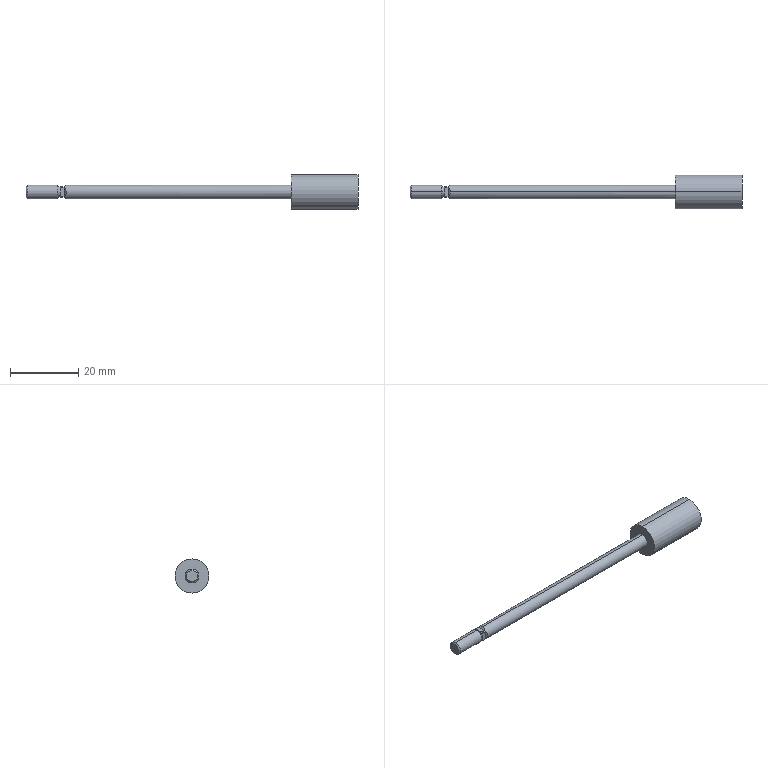Part | SolidWorks | features RefAxis 6, ICE 4, 3DProfileFeature 2, Revolution 1, Scale 1 | 1 solid | 30 faces | box 97.25 x 10 x 10 mm | volume 2498 mm3 | plane 16 | cylinder 8 | cone 6 | commonest cylinder face diameters 4 x4 3 x2 10 x2
STEP:
#1=CARTESIAN_POINT('',(126.058,0.000000064,5.));
#2=VERTEX_POINT('',#1);
#3=CARTESIAN_POINT('',(126.058,0.000000064,-5.));
#4=VERTEX_POINT('',#3);
#5=CARTESIAN_POINT('',(126.058,0.000000064,0.000001901));
#6=DIRECTION('',(-1.,0.,0.));
#7=DIRECTION('',(0.,0.,1.));
#8=AXIS2_PLACEMENT_3D('',#5,#6,#7);
#9=CIRCLE('',#8,5.);
#10=EDGE_CURVE('',#2,#4,#9,.T.);
#11=ORIENTED_EDGE('',*,*,#10,.T.);
#12=CARTESIAN_POINT('',(106.558,0.000000064,-5.));
#13=VERTEX_POINT('',#12);
#14=CARTESIAN_POINT('',(126.058,0.000000064,-5.));
#15=DIRECTION('',(-1.,0.,0.));
#16=VECTOR('',#15,1000.);
#17=LINE('',#14,#16);
#18=EDGE_CURVE('',#4,#13,#17,.T.);
#19=ORIENTED_EDGE('',*,*,#18,.T.);
#20=CARTESIAN_POINT('',(106.558,0.000000064,5.));
#21=VERTEX_POINT('',#20);
#22=CARTESIAN_POINT('',(106.558,0.000000064,0.000001901));
#23=DIRECTION('',(-1.,0.,0.));
#24=DIRECTION('',(0.,0.,1.));
#25=AXIS2_PLACEMENT_3D('',#22,#23,#24);
#26=CIRCLE('',#25,5.);
#27=EDGE_CURVE('',#21,#13,#26,.T.);
#28=ORIENTED_EDGE('',*,*,#27,.F.);
#29=CARTESIAN_POINT('',(126.058,0.000000064,5.));
#30=DIRECTION('',(-1.,0.,0.));
#31=VECTOR('',#30,1000.);
#32=LINE('',#29,#31);
#33=EDGE_CURVE('',#2,#21,#32,.T.);
#34=ORIENTED_EDGE('',*,*,#33,.F.);
#35=EDGE_LOOP('',(#11,#19,#28,#34));
#36=FACE_OUTER_BOUND('',#35,.T.);
#37=CARTESIAN_POINT('',(126.058,0.000000064,0.000001901));
#38=DIRECTION('',(-1.,0.,0.));
#39=DIRECTION('',(0.,0.,1.));
#40=AXIS2_PLACEMENT_3D('',#37,#38,#39);
#41=CYLINDRICAL_SURFACE('',#40,5.);
#42=ADVANCED_FACE('',(#36),#41,.T.);
#43=CARTESIAN_POINT('',(106.558,0.000000064,2.));
#44=VERTEX_POINT('',#43);
#45=CARTESIAN_POINT('',(106.558,0.000000064,-2.));
#46=VERTEX_POINT('',#45);
#47=CARTESIAN_POINT('',(106.558,0.000000064,0.000001901));
#48=DIRECTION('',(-1.,0.,0.));
#49=DIRECTION('',(0.,0.,1.));
#50=AXIS2_PLACEMENT_3D('',#47,#48,#49);
#51=CIRCLE('',#50,2.);
#52=EDGE_CURVE('',#44,#46,#51,.T.);
#53=ORIENTED_EDGE('',*,*,#52,.T.);
#54=CARTESIAN_POINT('',(40.558,0.000000064,-2.));
#55=VERTEX_POINT('',#54);
#56=CARTESIAN_POINT('',(126.058,0.000000064,-2.));
#57=DIRECTION('',(-1.,0.,0.));
#58=VECTOR('',#57,1000.);
#59=LINE('',#56,#58);
#60=EDGE_CURVE('',#46,#55,#59,.T.);
#61=ORIENTED_EDGE('',*,*,#60,.T.);
#62=CARTESIAN_POINT('',(40.058,1.323,-1.5));
#63=VERTEX_POINT('',#62);
#64=CARTESIAN_POINT('',(40.558,0.000000064,-2.));
#65=CARTESIAN_POINT('',(40.558,0.4926,-2.));
#66=CARTESIAN_POINT('',(40.384,0.9534,-1.826));
#67=CARTESIAN_POINT('',(40.058,1.323,-1.5));
#68=(BOUNDED_CURVE()B_SPLINE_CURVE(3,(#64,#65,#66,#67),.UNSPECIFIED.,.F.,.F.)B_SPLINE_CURVE_WITH_KNOTS((4,4),(3.142,3.864),.UNSPECIFIED.)CURVE()GEOMETRIC_REPRESENTATION_ITEM()RATIONAL_B_SPLINE_CURVE((1.,0.9569,0.9569,1.))REPRESENTATION_ITEM(''));
#69=EDGE_CURVE('',#55,#63,#68,.T.);
#70=ORIENTED_EDGE('',*,*,#69,.T.);
#71=CARTESIAN_POINT('',(39.183,1.323,-1.5));
#72=VERTEX_POINT('',#71);
#73=CARTESIAN_POINT('',(126.058,1.323,-1.5));
#74=DIRECTION('',(-1.,0.,0.));
#75=VECTOR('',#74,1000.);
#76=LINE('',#73,#75);
#77=EDGE_CURVE('',#63,#72,#76,.T.);
#78=ORIENTED_EDGE('',*,*,#77,.T.);
#79=CARTESIAN_POINT('',(39.183,1.5,-1.323));
#80=VERTEX_POINT('',#79);
#81=CARTESIAN_POINT('',(39.183,0.000000064,0.000001901));
#82=DIRECTION('',(-1.,0.,0.));
#83=DIRECTION('',(0.,0.,1.));
#84=AXIS2_PLACEMENT_3D('',#81,#82,#83);
#85=CIRCLE('',#84,2.);
#86=EDGE_CURVE('',#80,#72,#85,.T.);
#87=ORIENTED_EDGE('',*,*,#86,.F.);
#88=CARTESIAN_POINT('',(40.058,1.5,-1.323));
#89=VERTEX_POINT('',#88);
#90=CARTESIAN_POINT('',(126.058,1.5,-1.323));
#91=DIRECTION('',(1.,0.,0.));
#92=VECTOR('',#91,1000.);
#93=LINE('',#90,#92);
#94=EDGE_CURVE('',#80,#89,#93,.T.);
#95=ORIENTED_EDGE('',*,*,#94,.T.);
#96=CARTESIAN_POINT('',(40.058,1.5,1.323));
#97=VERTEX_POINT('',#96);
#98=CARTESIAN_POINT('',(40.058,1.5,-1.323));
#99=CARTESIAN_POINT('',(40.758,2.2,-0.5291));
#100=CARTESIAN_POINT('',(40.758,2.2,0.5292));
#101=CARTESIAN_POINT('',(40.058,1.5,1.323));
#102=(BOUNDED_CURVE()B_SPLINE_CURVE(3,(#98,#99,#100,#101),.UNSPECIFIED.,.F.,.F.)B_SPLINE_CURVE_WITH_KNOTS((4,4),(2.419,3.864),.UNSPECIFIED.)CURVE()GEOMETRIC_REPRESENTATION_ITEM()RATIONAL_B_SPLINE_CURVE((1.,0.8333,0.8333,1.))REPRESENTATION_ITEM(''));
#103=EDGE_CURVE('',#89,#97,#102,.T.);
#104=ORIENTED_EDGE('',*,*,#103,.T.);
#105=CARTESIAN_POINT('',(39.183,1.5,1.323));
#106=VERTEX_POINT('',#105);
#107=CARTESIAN_POINT('',(126.058,1.5,1.323));
#108=DIRECTION('',(-1.,0.,0.));
#109=VECTOR('',#108,1000.);
#110=LINE('',#107,#109);
#111=EDGE_CURVE('',#97,#106,#110,.T.);
#112=ORIENTED_EDGE('',*,*,#111,.T.);
#113=CARTESIAN_POINT('',(39.183,1.323,1.5));
#114=VERTEX_POINT('',#113);
#115=CARTESIAN_POINT('',(39.183,0.000000064,0.000001901));
#116=DIRECTION('',(-1.,0.,0.));
#117=DIRECTION('',(0.,0.,1.));
#118=AXIS2_PLACEMENT_3D('',#115,#116,#117);
#119=CIRCLE('',#118,2.);
#120=EDGE_CURVE('',#114,#106,#119,.T.);
#121=ORIENTED_EDGE('',*,*,#120,.F.);
#122=CARTESIAN_POINT('',(40.058,1.323,1.5));
#123=VERTEX_POINT('',#122);
#124=CARTESIAN_POINT('',(126.058,1.323,1.5));
#125=DIRECTION('',(1.,0.,0.));
#126=VECTOR('',#125,1000.);
#127=LINE('',#124,#126);
#128=EDGE_CURVE('',#114,#123,#127,.T.);
#129=ORIENTED_EDGE('',*,*,#128,.T.);
#130=CARTESIAN_POINT('',(40.558,0.000000064,2.));
#131=VERTEX_POINT('',#130);
#132=CARTESIAN_POINT('',(40.058,1.323,1.5));
#133=CARTESIAN_POINT('',(40.384,0.9534,1.826));
#134=CARTESIAN_POINT('',(40.558,0.4926,2.));
#135=CARTESIAN_POINT('',(40.558,0.000000064,2.));
#136=(BOUNDED_CURVE()B_SPLINE_CURVE(3,(#132,#133,#134,#135),.UNSPECIFIED.,.F.,.F.)B_SPLINE_CURVE_WITH_KNOTS((4,4),(2.419,3.142),.UNSPECIFIED.)CURVE()GEOMETRIC_REPRESENTATION_ITEM()RATIONAL_B_SPLINE_CURVE((1.,0.9569,0.9569,1.))REPRESENTATION_ITEM(''));
#137=EDGE_CURVE('',#123,#131,#136,.T.);
#138=ORIENTED_EDGE('',*,*,#137,.T.);
#139=CARTESIAN_POINT('',(126.058,0.000000064,2.));
#140=DIRECTION('',(-1.,0.,0.));
#141=VECTOR('',#140,1000.);
#142=LINE('',#139,#141);
#143=EDGE_CURVE('',#44,#131,#142,.T.);
#144=ORIENTED_EDGE('',*,*,#143,.F.);
#145=EDGE_LOOP('',(#53,#61,#70,#78,#87,#95,#104,#112,#121,#129,#138,#144));
#146=FACE_OUTER_BOUND('',#145,.T.);
#147=CARTESIAN_POINT('',(126.058,0.000000064,0.000001901));
#148=DIRECTION('',(-1.,0.,0.));
#149=DIRECTION('',(0.,0.,1.));
#150=AXIS2_PLACEMENT_3D('',#147,#148,#149);
#151=CYLINDRICAL_SURFACE('',#150,2.);
#152=ADVANCED_FACE('',(#146),#151,.T.);
#153=CARTESIAN_POINT('',(38.808,1.5,0.000001901));
#154=VERTEX_POINT('',#153);
#155=CARTESIAN_POINT('',(38.808,0.000000064,-1.5));
#156=VERTEX_POINT('',#155);
#157=CARTESIAN_POINT('',(38.808,0.000000064,0.000001901));
#158=DIRECTION('',(-1.,0.,0.));
#159=DIRECTION('',(0.,0.,1.));
#160=AXIS2_PLACEMENT_3D('',#157,#158,#159);
#161=CIRCLE('',#160,1.5);
#162=EDGE_CURVE('',#154,#156,#161,.T.);
#163=ORIENTED_EDGE('',*,*,#162,.T.);
#164=CARTESIAN_POINT('',(38.058,0.000000064,-1.5));
#165=VERTEX_POINT('',#164);
#166=CARTESIAN_POINT('',(126.058,0.000000064,-1.5));
#167=DIRECTION('',(-1.,0.,0.));
#168=VECTOR('',#167,1000.);
#169=LINE('',#166,#168);
#170=EDGE_CURVE('',#156,#165,#169,.T.);
#171=ORIENTED_EDGE('',*,*,#170,.T.);
#172=CARTESIAN_POINT('',(38.058,0.000000064,1.5));
#173=VERTEX_POINT('',#172);
#174=CARTESIAN_POINT('',(38.058,0.000000064,0.000001901));
#175=DIRECTION('',(-1.,0.,0.));
#176=DIRECTION('',(0.,0.,1.));
#177=AXIS2_PLACEMENT_3D('',#174,#175,#176);
#178=CIRCLE('',#177,1.5);
#179=EDGE_CURVE('',#173,#165,#178,.T.);
#180=ORIENTED_EDGE('',*,*,#179,.F.);
#181=CARTESIAN_POINT('',(38.808,0.000000064,1.5));
#182=VERTEX_POINT('',#181);
#183=CARTESIAN_POINT('',(126.058,0.000000064,1.5));
#184=DIRECTION('',(-1.,0.,0.));
#185=VECTOR('',#184,1000.);
#186=LINE('',#183,#185);
#187=EDGE_CURVE('',#182,#173,#186,.T.);
#188=ORIENTED_EDGE('',*,*,#187,.F.);
#189=CARTESIAN_POINT('',(38.808,0.000000064,0.000001901));
#190=DIRECTION('',(-1.,0.,0.));
#191=DIRECTION('',(0.,0.,1.));
#192=AXIS2_PLACEMENT_3D('',#189,#190,#191);
#193=CIRCLE('',#192,1.5);
#194=EDGE_CURVE('',#182,#154,#193,.T.);
#195=ORIENTED_EDGE('',*,*,#194,.T.);
#196=EDGE_LOOP('',(#163,#171,#180,#188,#195));
#197=FACE_OUTER_BOUND('',#196,.T.);
#198=CARTESIAN_POINT('',(126.058,0.000000064,0.000001901));
#199=DIRECTION('',(-1.,0.,0.));
#200=DIRECTION('',(0.,0.,1.));
#201=AXIS2_PLACEMENT_3D('',#198,#199,#200);
#202=CYLINDRICAL_SURFACE('',#201,1.5);
#203=ADVANCED_FACE('',(#197),#202,.T.);
#204=CARTESIAN_POINT('',(38.058,0.000000064,2.));
#205=VERTEX_POINT('',#204);
#206=CARTESIAN_POINT('',(38.058,0.000000064,-2.));
#207=VERTEX_POINT('',#206);
#208=CARTESIAN_POINT('',(38.058,0.000000064,0.000001901));
#209=DIRECTION('',(-1.,0.,0.));
#210=DIRECTION('',(0.,0.,1.));
#211=AXIS2_PLACEMENT_3D('',#208,#209,#210);
#212=CIRCLE('',#211,2.);
#213=EDGE_CURVE('',#205,#207,#212,.T.);
#214=ORIENTED_EDGE('',*,*,#213,.T.);
#215=CARTESIAN_POINT('',(29.192,0.000000064,-2.));
#216=VERTEX_POINT('',#215);
#217=CARTESIAN_POINT('',(126.058,0.000000064,-2.));
#218=DIRECTION('',(-1.,0.,0.));
#219=VECTOR('',#218,1000.);
#220=LINE('',#217,#219);
#221=EDGE_CURVE('',#207,#216,#220,.T.);
#222=ORIENTED_EDGE('',*,*,#221,.T.);
#223=CARTESIAN_POINT('',(29.192,0.000000064,2.));
#224=VERTEX_POINT('',#223);
#225=CARTESIAN_POINT('',(29.192,0.000000064,0.000001901));
#226=DIRECTION('',(-1.,0.,0.));
#227=DIRECTION('',(0.,0.,1.));
#228=AXIS2_PLACEMENT_3D('',#225,#226,#227);
#229=CIRCLE('',#228,2.);
#230=EDGE_CURVE('',#224,#216,#229,.T.);
#231=ORIENTED_EDGE('',*,*,#230,.F.);
#232=CARTESIAN_POINT('',(126.058,0.000000064,2.));
#233=DIRECTION('',(-1.,0.,0.));
#234=VECTOR('',#233,1000.);
#235=LINE('',#232,#234);
#236=EDGE_CURVE('',#205,#224,#235,.T.);
#237=ORIENTED_EDGE('',*,*,#236,.F.);
#238=EDGE_LOOP('',(#214,#222,#231,#237));
#239=FACE_OUTER_BOUND('',#238,.T.);
#240=CARTESIAN_POINT('',(126.058,0.000000064,0.000001901));
#241=DIRECTION('',(-1.,0.,0.));
#242=DIRECTION('',(0.,0.,1.));
#243=AXIS2_PLACEMENT_3D('',#240,#241,#242);
#244=CYLINDRICAL_SURFACE('',#243,2.);
#245=ADVANCED_FACE('',(#239),#244,.T.);
#246=CARTESIAN_POINT('',(28.808,0.000000064,1.617));
#247=VERTEX_POINT('',#246);
#248=CARTESIAN_POINT('',(28.808,0.000000064,-1.616));
#249=VERTEX_POINT('',#248);
#250=CARTESIAN_POINT('',(28.808,0.000000064,0.000001901));
#251=DIRECTION('',(-1.,0.,0.));
#252=DIRECTION('',(0.,0.,1.));
#253=AXIS2_PLACEMENT_3D('',#250,#251,#252);
#254=CIRCLE('',#253,1.617);
#255=EDGE_CURVE('',#247,#249,#254,.T.);
#256=ORIENTED_EDGE('',*,*,#255,.F.);
#257=CARTESIAN_POINT('',(29.192,0.000000064,2.));
#258=DIRECTION('',(0.7071,0.,0.7071));
#259=VECTOR('',#258,1000.);
#260=LINE('',#257,#259);
#261=EDGE_CURVE('',#247,#224,#260,.T.);
#262=ORIENTED_EDGE('',*,*,#261,.T.);
#263=ORIENTED_EDGE('',*,*,#230,.T.);
#264=CARTESIAN_POINT('',(29.192,0.000000064,-2.));
#265=DIRECTION('',(0.7071,0.,-0.7071));
#266=VECTOR('',#265,1000.);
#267=LINE('',#264,#266);
#268=EDGE_CURVE('',#249,#216,#267,.T.);
#269=ORIENTED_EDGE('',*,*,#268,.F.);
#270=EDGE_LOOP('',(#256,#262,#263,#269));
#271=FACE_OUTER_BOUND('',#270,.T.);
#272=CARTESIAN_POINT('',(29.192,0.000000064,0.000001901));
#273=DIRECTION('',(1.,0.,0.));
#274=DIRECTION('',(0.,0.,-1.));
#275=AXIS2_PLACEMENT_3D('',#272,#273,#274);
#276=CONICAL_SURFACE('',#275,2.,0.7854);
#277=ADVANCED_FACE('',(#271),#276,.T.);
#278=CARTESIAN_POINT('',(38.808,-1.5,0.625));
#279=VERTEX_POINT('',#278);
#280=CARTESIAN_POINT('',(38.808,-0.625,1.5));
#281=VERTEX_POINT('',#280);
#282=CARTESIAN_POINT('',(38.808,0.000000064,0.000001901));
#283=DIRECTION('',(-1.,0.,0.));
#284=DIRECTION('',(0.,0.,1.));
#285=AXIS2_PLACEMENT_3D('',#282,#283,#284);
#286=CIRCLE('',#285,1.625);
#287=EDGE_CURVE('',#279,#281,#286,.T.);
#288=ORIENTED_EDGE('',*,*,#287,.T.);
#289=CARTESIAN_POINT('',(38.808,-2.,1.5));
#290=DIRECTION('',(0.,1.,0.));
#291=VECTOR('',#290,1000.);
#292=LINE('',#289,#291);
#293=EDGE_CURVE('',#281,#182,#292,.T.);
#294=ORIENTED_EDGE('',*,*,#293,.T.);
#295=CARTESIAN_POINT('',(38.808,-1.5,0.000001901));
#296=VERTEX_POINT('',#295);
#297=CARTESIAN_POINT('',(38.808,0.000000064,0.000001901));
#298=DIRECTION('',(-1.,0.,0.));
#299=DIRECTION('',(0.,0.,1.));
#300=AXIS2_PLACEMENT_3D('',#297,#298,#299);
#301=CIRCLE('',#300,1.5);
#302=EDGE_CURVE('',#296,#182,#301,.T.);
#303=ORIENTED_EDGE('',*,*,#302,.F.);
#304=CARTESIAN_POINT('',(38.808,-1.5,-2.));
#305=DIRECTION('',(0.,0.,1.));
#306=VECTOR('',#305,1000.);
#307=LINE('',#304,#306);
#308=EDGE_CURVE('',#296,#279,#307,.T.);
#309=ORIENTED_EDGE('',*,*,#308,.T.);
#310=EDGE_LOOP('',(#288,#294,#303,#309));
#311=FACE_OUTER_BOUND('',#310,.T.);
#312=CARTESIAN_POINT('',(38.808,1.5,0.000001901));
#313=DIRECTION('',(1.,0.,0.));
#314=DIRECTION('',(0.,0.,-1.));
#315=AXIS2_PLACEMENT_3D('',#312,#313,#314);
#316=PLANE('',#315);
#317=ADVANCED_FACE('',(#311),#316,.F.);
#318=CARTESIAN_POINT('',(39.183,-1.5,1.323));
#319=VERTEX_POINT('',#318);
#320=CARTESIAN_POINT('',(39.183,-1.323,1.5));
#321=VERTEX_POINT('',#320);
#322=CARTESIAN_POINT('',(39.183,0.000000064,0.000001901));
#323=DIRECTION('',(-1.,0.,0.));
#324=DIRECTION('',(0.,0.,1.));
#325=AXIS2_PLACEMENT_3D('',#322,#323,#324);
#326=CIRCLE('',#325,2.);
#327=EDGE_CURVE('',#319,#321,#326,.T.);
#328=ORIENTED_EDGE('',*,*,#327,.T.);
#329=CARTESIAN_POINT('',(39.183,-1.323,1.5));
#330=CARTESIAN_POINT('',(39.037,-1.103,1.5));
#331=CARTESIAN_POINT('',(38.903,-0.8715,1.5));
#332=CARTESIAN_POINT('',(38.808,-0.625,1.5));
#333=B_SPLINE_CURVE_WITH_KNOTS('',3,(#329,#330,#331,#332),.UNSPECIFIED.,.F.,.F.,(4,4),(0.002581,0.003375),.UNSPECIFIED.);
#334=EDGE_CURVE('',#321,#281,#333,.T.);
#335=ORIENTED_EDGE('',*,*,#334,.T.);
#336=ORIENTED_EDGE('',*,*,#287,.F.);
#337=CARTESIAN_POINT('',(38.808,-1.5,0.625));
#338=CARTESIAN_POINT('',(38.903,-1.5,0.8718));
#339=CARTESIAN_POINT('',(39.037,-1.5,1.102));
#340=CARTESIAN_POINT('',(39.183,-1.5,1.323));
#341=B_SPLINE_CURVE_WITH_KNOTS('',3,(#337,#338,#339,#340),.UNSPECIFIED.,.F.,.F.,(4,4),(0.005782,0.006571),.UNSPECIFIED.);
#342=EDGE_CURVE('',#279,#319,#341,.T.);
#343=ORIENTED_EDGE('',*,*,#342,.T.);
#344=EDGE_LOOP('',(#328,#335,#336,#343));
#345=FACE_OUTER_BOUND('',#344,.T.);
#346=CARTESIAN_POINT('',(39.183,0.000000064,0.000001901));
#347=DIRECTION('',(1.,0.,0.));
#348=DIRECTION('',(0.,0.,-1.));
#349=AXIS2_PLACEMENT_3D('',#346,#347,#348);
#350=CONICAL_SURFACE('',#349,2.,0.7854);
#351=ADVANCED_FACE('',(#345),#350,.T.);
#352=CARTESIAN_POINT('',(38.808,1.5,-0.625));
#353=VERTEX_POINT('',#352);
#354=CARTESIAN_POINT('',(38.808,0.625,-1.5));
#355=VERTEX_POINT('',#354);
#356=CARTESIAN_POINT('',(38.808,0.000000064,0.000001901));
#357=DIRECTION('',(-1.,0.,0.));
#358=DIRECTION('',(0.,0.,1.));
#359=AXIS2_PLACEMENT_3D('',#356,#357,#358);
#360=CIRCLE('',#359,1.625);
#361=EDGE_CURVE('',#353,#355,#360,.T.);
#362=ORIENTED_EDGE('',*,*,#361,.T.);
#363=CARTESIAN_POINT('',(38.808,-2.,-1.5));
#364=DIRECTION('',(0.,1.,0.));
#365=VECTOR('',#364,1000.);
#366=LINE('',#363,#365);
#367=EDGE_CURVE('',#156,#355,#366,.T.);
#368=ORIENTED_EDGE('',*,*,#367,.F.);
#369=ORIENTED_EDGE('',*,*,#162,.F.);
#370=CARTESIAN_POINT('',(38.808,1.5,-2.));
#371=DIRECTION('',(0.,0.,1.));
#372=VECTOR('',#371,1000.);
#373=LINE('',#370,#372);
#374=EDGE_CURVE('',#353,#154,#373,.T.);
#375=ORIENTED_EDGE('',*,*,#374,.F.);
#376=EDGE_LOOP('',(#362,#368,#369,#375));
#377=FACE_OUTER_BOUND('',#376,.T.);
#378=CARTESIAN_POINT('',(38.808,1.5,0.000001901));
#379=DIRECTION('',(1.,0.,0.));
#380=DIRECTION('',(0.,0.,-1.));
#381=AXIS2_PLACEMENT_3D('',#378,#379,#380);
#382=PLANE('',#381);
#383=ADVANCED_FACE('',(#377),#382,.F.);
#384=ORIENTED_EDGE('',*,*,#86,.T.);
#385=CARTESIAN_POINT('',(39.183,1.323,-1.5));
#386=CARTESIAN_POINT('',(39.037,1.103,-1.5));
#387=CARTESIAN_POINT('',(38.903,0.8715,-1.5));
#388=CARTESIAN_POINT('',(38.808,0.625,-1.5));
#389=B_SPLINE_CURVE_WITH_KNOTS('',3,(#385,#386,#387,#388),.UNSPECIFIED.,.F.,.F.,(4,4),(0.002581,0.003375),.UNSPECIFIED.);
#390=EDGE_CURVE('',#72,#355,#389,.T.);
#391=ORIENTED_EDGE('',*,*,#390,.T.);
#392=ORIENTED_EDGE('',*,*,#361,.F.);
#393=CARTESIAN_POINT('',(38.808,1.5,-0.625));
#394=CARTESIAN_POINT('',(38.903,1.5,-0.8718));
#395=CARTESIAN_POINT('',(39.037,1.5,-1.102));
#396=CARTESIAN_POINT('',(39.183,1.5,-1.323));
#397=B_SPLINE_CURVE_WITH_KNOTS('',3,(#393,#394,#395,#396),.UNSPECIFIED.,.F.,.F.,(4,4),(0.005782,0.006571),.UNSPECIFIED.);
#398=EDGE_CURVE('',#353,#80,#397,.T.);
#399=ORIENTED_EDGE('',*,*,#398,.T.);
#400=EDGE_LOOP('',(#384,#391,#392,#399));
#401=FACE_OUTER_BOUND('',#400,.T.);
#402=CARTESIAN_POINT('',(39.183,0.000000064,0.000001901));
#403=DIRECTION('',(1.,0.,0.));
#404=DIRECTION('',(0.,0.,-1.));
#405=AXIS2_PLACEMENT_3D('',#402,#403,#404);
#406=CONICAL_SURFACE('',#405,2.,0.7854);
#407=ADVANCED_FACE('',(#401),#406,.T.);
#408=CARTESIAN_POINT('',(38.808,0.000000064,0.000001901));
#409=DIRECTION('',(-1.,0.,0.));
#410=DIRECTION('',(0.,0.,1.));
#411=AXIS2_PLACEMENT_3D('',#408,#409,#410);
#412=CIRCLE('',#411,1.5);
#413=EDGE_CURVE('',#156,#296,#412,.T.);
#414=ORIENTED_EDGE('',*,*,#413,.F.);
#415=CARTESIAN_POINT('',(38.808,-0.625,-1.5));
#416=VERTEX_POINT('',#415);
#417=CARTESIAN_POINT('',(38.808,-2.,-1.5));
#418=DIRECTION('',(0.,1.,0.));
#419=VECTOR('',#418,1000.);
#420=LINE('',#417,#419);
#421=EDGE_CURVE('',#416,#156,#420,.T.);
#422=ORIENTED_EDGE('',*,*,#421,.F.);
#423=CARTESIAN_POINT('',(38.808,-1.5,-0.625));
#424=VERTEX_POINT('',#423);
#425=CARTESIAN_POINT('',(38.808,0.000000064,0.000001901));
#426=DIRECTION('',(-1.,0.,0.));
#427=DIRECTION('',(0.,0.,1.));
#428=AXIS2_PLACEMENT_3D('',#425,#426,#427);
#429=CIRCLE('',#428,1.625);
#430=EDGE_CURVE('',#416,#424,#429,.T.);
#431=ORIENTED_EDGE('',*,*,#430,.T.);
#432=CARTESIAN_POINT('',(38.808,-1.5,-2.));
#433=DIRECTION('',(0.,0.,1.));
#434=VECTOR('',#433,1000.);
#435=LINE('',#432,#434);
#436=EDGE_CURVE('',#424,#296,#435,.T.);
#437=ORIENTED_EDGE('',*,*,#436,.T.);
#438=EDGE_LOOP('',(#414,#422,#431,#437));
#439=FACE_OUTER_BOUND('',#438,.T.);
#440=CARTESIAN_POINT('',(38.808,1.5,0.000001901));
#441=DIRECTION('',(1.,0.,0.));
#442=DIRECTION('',(0.,0.,-1.));
#443=AXIS2_PLACEMENT_3D('',#440,#441,#442);
#444=PLANE('',#443);
#445=ADVANCED_FACE('',(#439),#444,.F.);
#446=ORIENTED_EDGE('',*,*,#430,.F.);
#447=CARTESIAN_POINT('',(39.183,-1.323,-1.5));
#448=VERTEX_POINT('',#447);
#449=CARTESIAN_POINT('',(38.808,-0.625,-1.5));
#450=CARTESIAN_POINT('',(38.904,-0.8751,-1.5));
#451=CARTESIAN_POINT('',(39.038,-1.103,-1.5));
#452=CARTESIAN_POINT('',(39.183,-1.323,-1.5));
#453=B_SPLINE_CURVE_WITH_KNOTS('',3,(#449,#450,#451,#452),.UNSPECIFIED.,.F.,.F.,(4,4),(0.004656,0.005455),.UNSPECIFIED.);
#454=EDGE_CURVE('',#416,#448,#453,.T.);
#455=ORIENTED_EDGE('',*,*,#454,.T.);
#456=CARTESIAN_POINT('',(39.183,-1.5,-1.323));
#457=VERTEX_POINT('',#456);
#458=CARTESIAN_POINT('',(39.183,0.000000064,0.000001901));
#459=DIRECTION('',(-1.,0.,0.));
#460=DIRECTION('',(0.,0.,1.));
#461=AXIS2_PLACEMENT_3D('',#458,#459,#460);
#462=CIRCLE('',#461,2.);
#463=EDGE_CURVE('',#448,#457,#462,.T.);
#464=ORIENTED_EDGE('',*,*,#463,.T.);
#465=CARTESIAN_POINT('',(39.183,-1.5,-1.323));
#466=CARTESIAN_POINT('',(39.111,-1.5,-1.213));
#467=CARTESIAN_POINT('',(39.042,-1.5,-1.102));
#468=CARTESIAN_POINT('',(38.914,-1.5,-0.87));
#469=CARTESIAN_POINT('',(38.856,-1.5,-0.7492));
#470=CARTESIAN_POINT('',(38.808,-1.5,-0.625));
#471=B_SPLINE_CURVE_WITH_KNOTS('',3,(#465,#466,#467,#468,#469,#470),.UNSPECIFIED.,.F.,.F.,(4,2,4),(0.003721,0.004116,0.004511),.UNSPECIFIED.);
#472=EDGE_CURVE('',#457,#424,#471,.T.);
#473=ORIENTED_EDGE('',*,*,#472,.T.);
#474=EDGE_LOOP('',(#446,#455,#464,#473));
#475=FACE_OUTER_BOUND('',#474,.T.);
#476=CARTESIAN_POINT('',(39.183,0.000000064,0.000001901));
#477=DIRECTION('',(1.,0.,0.));
#478=DIRECTION('',(0.,0.,-1.));
#479=AXIS2_PLACEMENT_3D('',#476,#477,#478);
#480=CONICAL_SURFACE('',#479,2.,0.7854);
#481=ADVANCED_FACE('',(#475),#480,.T.);
#482=CARTESIAN_POINT('',(28.808,0.000000064,0.000001901));
#483=DIRECTION('',(-1.,0.,0.));
#484=DIRECTION('',(0.,0.,1.));
#485=AXIS2_PLACEMENT_3D('',#482,#483,#484);
#486=CIRCLE('',#485,1.617);
#487=EDGE_CURVE('',#249,#247,#486,.T.);
#488=ORIENTED_EDGE('',*,*,#487,.T.);
#489=ORIENTED_EDGE('',*,*,#255,.T.);
#490=EDGE_LOOP('',(#488,#489));
#491=FACE_OUTER_BOUND('',#490,.T.);
#492=CARTESIAN_POINT('',(28.808,0.000000064,0.000001901));
#493=DIRECTION('',(1.,0.,0.));
#494=DIRECTION('',(0.,0.,-1.));
#495=AXIS2_PLACEMENT_3D('',#492,#493,#494);
#496=PLANE('',#495);
#497=ADVANCED_FACE('',(#491),#496,.F.);
#498=ORIENTED_EDGE('',*,*,#261,.F.);
#499=ORIENTED_EDGE('',*,*,#487,.F.);
#500=ORIENTED_EDGE('',*,*,#268,.T.);
#501=CARTESIAN_POINT('',(29.192,0.000000064,0.000001901));
#502=DIRECTION('',(-1.,0.,0.));
#503=DIRECTION('',(0.,0.,1.));
#504=AXIS2_PLACEMENT_3D('',#501,#502,#503);
#505=CIRCLE('',#504,2.);
#506=EDGE_CURVE('',#216,#224,#505,.T.);
#507=ORIENTED_EDGE('',*,*,#506,.T.);
#508=EDGE_LOOP('',(#498,#499,#500,#507));
#509=FACE_OUTER_BOUND('',#508,.T.);
#510=CARTESIAN_POINT('',(29.192,0.000000064,0.000001901));
#511=DIRECTION('',(1.,0.,0.));
#512=DIRECTION('',(0.,0.,-1.));
#513=AXIS2_PLACEMENT_3D('',#510,#511,#512);
#514=CONICAL_SURFACE('',#513,2.,0.7854);
#515=ADVANCED_FACE('',(#509),#514,.T.);
#516=ORIENTED_EDGE('',*,*,#221,.F.);
#517=CARTESIAN_POINT('',(38.058,0.000000064,0.000001901));
#518=DIRECTION('',(-1.,0.,0.));
#519=DIRECTION('',(0.,0.,1.));
#520=AXIS2_PLACEMENT_3D('',#517,#518,#519);
#521=CIRCLE('',#520,2.);
#522=EDGE_CURVE('',#207,#205,#521,.T.);
#523=ORIENTED_EDGE('',*,*,#522,.T.);
#524=ORIENTED_EDGE('',*,*,#236,.T.);
#525=ORIENTED_EDGE('',*,*,#506,.F.);
#526=EDGE_LOOP('',(#516,#523,#524,#525));
#527=FACE_OUTER_BOUND('',#526,.T.);
#528=CARTESIAN_POINT('',(126.058,0.000000064,0.000001901));
#529=DIRECTION('',(-1.,0.,0.));
#530=DIRECTION('',(0.,0.,1.));
#531=AXIS2_PLACEMENT_3D('',#528,#529,#530);
#532=CYLINDRICAL_SURFACE('',#531,2.);
#533=ADVANCED_FACE('',(#527),#532,.T.);
#534=ORIENTED_EDGE('',*,*,#213,.F.);
#535=ORIENTED_EDGE('',*,*,#522,.F.);
#536=EDGE_LOOP('',(#534,#535));
#537=FACE_OUTER_BOUND('',#536,.T.);
#538=ORIENTED_EDGE('',*,*,#179,.T.);
#539=CARTESIAN_POINT('',(38.058,0.000000064,0.000001901));
#540=DIRECTION('',(-1.,0.,0.));
#541=DIRECTION('',(0.,0.,1.));
#542=AXIS2_PLACEMENT_3D('',#539,#540,#541);
#543=CIRCLE('',#542,1.5);
#544=EDGE_CURVE('',#165,#173,#543,.T.);
#545=ORIENTED_EDGE('',*,*,#544,.T.);
#546=EDGE_LOOP('',(#538,#545));
#547=FACE_BOUND('',#546,.T.);
#548=CARTESIAN_POINT('',(38.058,2.,0.000001901));
#549=DIRECTION('',(-1.,0.,0.));
#550=DIRECTION('',(0.,0.,1.));
#551=AXIS2_PLACEMENT_3D('',#548,#549,#550);
#552=PLANE('',#551);
#553=ADVANCED_FACE('',(#537,#547),#552,.F.);
#554=ORIENTED_EDGE('',*,*,#170,.F.);
#555=ORIENTED_EDGE('',*,*,#413,.T.);
#556=ORIENTED_EDGE('',*,*,#302,.T.);
#557=ORIENTED_EDGE('',*,*,#187,.T.);
#558=ORIENTED_EDGE('',*,*,#544,.F.);
#559=EDGE_LOOP('',(#554,#555,#556,#557,#558));
#560=FACE_OUTER_BOUND('',#559,.T.);
#561=CARTESIAN_POINT('',(126.058,0.000000064,0.000001901));
#562=DIRECTION('',(-1.,0.,0.));
#563=DIRECTION('',(0.,0.,1.));
#564=AXIS2_PLACEMENT_3D('',#561,#562,#563);
#565=CYLINDRICAL_SURFACE('',#564,1.5);
#566=ADVANCED_FACE('',(#560),#565,.T.);
#567=ORIENTED_EDGE('',*,*,#194,.F.);
#568=CARTESIAN_POINT('',(38.808,0.625,1.5));
#569=VERTEX_POINT('',#568);
#570=CARTESIAN_POINT('',(38.808,-2.,1.5));
#571=DIRECTION('',(0.,1.,0.));
#572=VECTOR('',#571,1000.);
#573=LINE('',#570,#572);
#574=EDGE_CURVE('',#182,#569,#573,.T.);
#575=ORIENTED_EDGE('',*,*,#574,.T.);
#576=CARTESIAN_POINT('',(38.808,1.5,0.625));
#577=VERTEX_POINT('',#576);
#578=CARTESIAN_POINT('',(38.808,0.000000064,0.000001901));
#579=DIRECTION('',(-1.,0.,0.));
#580=DIRECTION('',(0.,0.,1.));
#581=AXIS2_PLACEMENT_3D('',#578,#579,#580);
#582=CIRCLE('',#581,1.625);
#583=EDGE_CURVE('',#569,#577,#582,.T.);
#584=ORIENTED_EDGE('',*,*,#583,.T.);
#585=CARTESIAN_POINT('',(38.808,1.5,-2.));
#586=DIRECTION('',(0.,0.,1.));
#587=VECTOR('',#586,1000.);
#588=LINE('',#585,#587);
#589=EDGE_CURVE('',#154,#577,#588,.T.);
#590=ORIENTED_EDGE('',*,*,#589,.F.);
#591=EDGE_LOOP('',(#567,#575,#584,#590));
#592=FACE_OUTER_BOUND('',#591,.T.);
#593=CARTESIAN_POINT('',(38.808,1.5,0.000001901));
#594=DIRECTION('',(1.,0.,0.));
#595=DIRECTION('',(0.,0.,-1.));
#596=AXIS2_PLACEMENT_3D('',#593,#594,#595);
#597=PLANE('',#596);
#598=ADVANCED_FACE('',(#592),#597,.F.);
#599=ORIENTED_EDGE('',*,*,#583,.F.);
#600=CARTESIAN_POINT('',(38.808,0.625,1.5));
#601=CARTESIAN_POINT('',(38.904,0.8751,1.5));
#602=CARTESIAN_POINT('',(39.038,1.103,1.5));
#603=CARTESIAN_POINT('',(39.183,1.323,1.5));
#604=B_SPLINE_CURVE_WITH_KNOTS('',3,(#600,#601,#602,#603),.UNSPECIFIED.,.F.,.F.,(4,4),(0.004656,0.005455),.UNSPECIFIED.);
#605=EDGE_CURVE('',#569,#114,#604,.T.);
#606=ORIENTED_EDGE('',*,*,#605,.T.);
#607=ORIENTED_EDGE('',*,*,#120,.T.);
#608=CARTESIAN_POINT('',(39.183,1.5,1.323));
#609=CARTESIAN_POINT('',(39.111,1.5,1.213));
#610=CARTESIAN_POINT('',(39.042,1.5,1.102));
#611=CARTESIAN_POINT('',(38.914,1.5,0.87));
#612=CARTESIAN_POINT('',(38.856,1.5,0.7492));
#613=CARTESIAN_POINT('',(38.808,1.5,0.625));
#614=B_SPLINE_CURVE_WITH_KNOTS('',3,(#608,#609,#610,#611,#612,#613),.UNSPECIFIED.,.F.,.F.,(4,2,4),(0.003721,0.004116,0.004511),.UNSPECIFIED.);
#615=EDGE_CURVE('',#106,#577,#614,.T.);
#616=ORIENTED_EDGE('',*,*,#615,.T.);
#617=EDGE_LOOP('',(#599,#606,#607,#616));
#618=FACE_OUTER_BOUND('',#617,.T.);
#619=CARTESIAN_POINT('',(39.183,0.000000064,0.000001901));
#620=DIRECTION('',(1.,0.,0.));
#621=DIRECTION('',(0.,0.,-1.));
#622=AXIS2_PLACEMENT_3D('',#619,#620,#621);
#623=CONICAL_SURFACE('',#622,2.,0.7854);
#624=ADVANCED_FACE('',(#618),#623,.T.);
#625=ORIENTED_EDGE('',*,*,#60,.F.);
#626=CARTESIAN_POINT('',(106.558,0.000000064,0.000001901));
#627=DIRECTION('',(-1.,0.,0.));
#628=DIRECTION('',(0.,0.,1.));
#629=AXIS2_PLACEMENT_3D('',#626,#627,#628);
#630=CIRCLE('',#629,2.);
#631=EDGE_CURVE('',#46,#44,#630,.T.);
#632=ORIENTED_EDGE('',*,*,#631,.T.);
#633=ORIENTED_EDGE('',*,*,#143,.T.);
#634=CARTESIAN_POINT('',(40.058,-1.323,1.5));
#635=VERTEX_POINT('',#634);
#636=CARTESIAN_POINT('',(40.558,0.000000064,2.));
#637=CARTESIAN_POINT('',(40.558,-0.4926,2.));
#638=CARTESIAN_POINT('',(40.384,-0.9534,1.826));
#639=CARTESIAN_POINT('',(40.058,-1.323,1.5));
#640=(BOUNDED_CURVE()B_SPLINE_CURVE(3,(#636,#637,#638,#639),.UNSPECIFIED.,.F.,.F.)B_SPLINE_CURVE_WITH_KNOTS((4,4),(3.142,3.864),.UNSPECIFIED.)CURVE()GEOMETRIC_REPRESENTATION_ITEM()RATIONAL_B_SPLINE_CURVE((1.,0.9569,0.9569,1.))REPRESENTATION_ITEM(''));
#641=EDGE_CURVE('',#131,#635,#640,.T.);
#642=ORIENTED_EDGE('',*,*,#641,.T.);
#643=CARTESIAN_POINT('',(126.058,-1.323,1.5));
#644=DIRECTION('',(-1.,0.,0.));
#645=VECTOR('',#644,1000.);
#646=LINE('',#643,#645);
#647=EDGE_CURVE('',#635,#321,#646,.T.);
#648=ORIENTED_EDGE('',*,*,#647,.T.);
#649=ORIENTED_EDGE('',*,*,#327,.F.);
#650=CARTESIAN_POINT('',(40.058,-1.5,1.323));
#651=VERTEX_POINT('',#650);
#652=CARTESIAN_POINT('',(126.058,-1.5,1.323));
#653=DIRECTION('',(1.,0.,0.));
#654=VECTOR('',#653,1000.);
#655=LINE('',#652,#654);
#656=EDGE_CURVE('',#319,#651,#655,.T.);
#657=ORIENTED_EDGE('',*,*,#656,.T.);
#658=CARTESIAN_POINT('',(40.058,-1.5,-1.323));
#659=VERTEX_POINT('',#658);
#660=CARTESIAN_POINT('',(40.058,-1.5,1.323));
#661=CARTESIAN_POINT('',(40.758,-2.2,0.5292));
#662=CARTESIAN_POINT('',(40.758,-2.2,-0.5291));
#663=CARTESIAN_POINT('',(40.058,-1.5,-1.323));
#664=(BOUNDED_CURVE()B_SPLINE_CURVE(3,(#660,#661,#662,#663),.UNSPECIFIED.,.F.,.F.)B_SPLINE_CURVE_WITH_KNOTS((4,4),(2.419,3.864),.UNSPECIFIED.)CURVE()GEOMETRIC_REPRESENTATION_ITEM()RATIONAL_B_SPLINE_CURVE((1.,0.8333,0.8333,1.))REPRESENTATION_ITEM(''));
#665=EDGE_CURVE('',#651,#659,#664,.T.);
#666=ORIENTED_EDGE('',*,*,#665,.T.);
#667=CARTESIAN_POINT('',(126.058,-1.5,-1.323));
#668=DIRECTION('',(-1.,0.,0.));
#669=VECTOR('',#668,1000.);
#670=LINE('',#667,#669);
#671=EDGE_CURVE('',#659,#457,#670,.T.);
#672=ORIENTED_EDGE('',*,*,#671,.T.);
#673=ORIENTED_EDGE('',*,*,#463,.F.);
#674=CARTESIAN_POINT('',(40.058,-1.323,-1.5));
#675=VERTEX_POINT('',#674);
#676=CARTESIAN_POINT('',(126.058,-1.323,-1.5));
#677=DIRECTION('',(1.,0.,0.));
#678=VECTOR('',#677,1000.);
#679=LINE('',#676,#678);
#680=EDGE_CURVE('',#448,#675,#679,.T.);
#681=ORIENTED_EDGE('',*,*,#680,.T.);
#682=CARTESIAN_POINT('',(40.058,-1.323,-1.5));
#683=CARTESIAN_POINT('',(40.384,-0.9534,-1.826));
#684=CARTESIAN_POINT('',(40.558,-0.4926,-2.));
#685=CARTESIAN_POINT('',(40.558,0.000000064,-2.));
#686=(BOUNDED_CURVE()B_SPLINE_CURVE(3,(#682,#683,#684,#685),.UNSPECIFIED.,.F.,.T.)B_SPLINE_CURVE_WITH_KNOTS((4,4),(2.419,3.142),.UNSPECIFIED.)CURVE()GEOMETRIC_REPRESENTATION_ITEM()RATIONAL_B_SPLINE_CURVE((1.,0.9569,0.9569,1.))REPRESENTATION_ITEM(''));
#687=EDGE_CURVE('',#675,#55,#686,.T.);
#688=ORIENTED_EDGE('',*,*,#687,.T.);
#689=EDGE_LOOP('',(#625,#632,#633,#642,#648,#649,#657,#666,#672,#673,#681,#688));
#690=FACE_OUTER_BOUND('',#689,.T.);
#691=CARTESIAN_POINT('',(126.058,0.000000064,0.000001901));
#692=DIRECTION('',(-1.,0.,0.));
#693=DIRECTION('',(0.,0.,1.));
#694=AXIS2_PLACEMENT_3D('',#691,#692,#693);
#695=CYLINDRICAL_SURFACE('',#694,2.);
#696=ADVANCED_FACE('',(#690),#695,.T.);
#697=ORIENTED_EDGE('',*,*,#52,.F.);
#698=ORIENTED_EDGE('',*,*,#631,.F.);
#699=EDGE_LOOP('',(#697,#698));
#700=FACE_BOUND('',#699,.T.);
#701=ORIENTED_EDGE('',*,*,#27,.T.);
#702=CARTESIAN_POINT('',(106.558,0.000000064,0.000001901));
#703=DIRECTION('',(-1.,0.,0.));
#704=DIRECTION('',(0.,0.,1.));
#705=AXIS2_PLACEMENT_3D('',#702,#703,#704);
#706=CIRCLE('',#705,5.);
#707=EDGE_CURVE('',#13,#21,#706,.T.);
#708=ORIENTED_EDGE('',*,*,#707,.T.);
#709=EDGE_LOOP('',(#701,#708));
#710=FACE_OUTER_BOUND('',#709,.T.);
#711=CARTESIAN_POINT('',(106.558,2.,0.000001901));
#712=DIRECTION('',(1.,0.,0.));
#713=DIRECTION('',(0.,0.,-1.));
#714=AXIS2_PLACEMENT_3D('',#711,#712,#713);
#715=PLANE('',#714);
#716=ADVANCED_FACE('',(#700,#710),#715,.F.);
#717=ORIENTED_EDGE('',*,*,#18,.F.);
#718=CARTESIAN_POINT('',(126.058,0.000000064,0.000001901));
#719=DIRECTION('',(-1.,0.,0.));
#720=DIRECTION('',(0.,0.,1.));
#721=AXIS2_PLACEMENT_3D('',#718,#719,#720);
#722=CIRCLE('',#721,5.);
#723=EDGE_CURVE('',#4,#2,#722,.T.);
#724=ORIENTED_EDGE('',*,*,#723,.T.);
#725=ORIENTED_EDGE('',*,*,#33,.T.);
#726=ORIENTED_EDGE('',*,*,#707,.F.);
#727=EDGE_LOOP('',(#717,#724,#725,#726));
#728=FACE_OUTER_BOUND('',#727,.T.);
#729=CARTESIAN_POINT('',(126.058,0.000000064,0.000001901));
#730=DIRECTION('',(-1.,0.,0.));
#731=DIRECTION('',(0.,0.,1.));
#732=AXIS2_PLACEMENT_3D('',#729,#730,#731);
#733=CYLINDRICAL_SURFACE('',#732,5.);
#734=ADVANCED_FACE('',(#728),#733,.T.);
#735=ORIENTED_EDGE('',*,*,#10,.F.);
#736=ORIENTED_EDGE('',*,*,#723,.F.);
#737=EDGE_LOOP('',(#735,#736));
#738=FACE_OUTER_BOUND('',#737,.T.);
#739=CARTESIAN_POINT('',(126.058,5.,0.000001901));
#740=DIRECTION('',(-1.,0.,0.));
#741=DIRECTION('',(0.,0.,1.));
#742=AXIS2_PLACEMENT_3D('',#739,#740,#741);
#743=PLANE('',#742);
#744=ADVANCED_FACE('',(#738),#743,.F.);
#745=CARTESIAN_POINT('',(40.058,1.5,-2.));
#746=DIRECTION('',(0.,0.,1.));
#747=VECTOR('',#746,1000.);
#748=LINE('',#745,#747);
#749=EDGE_CURVE('',#89,#97,#748,.T.);
#750=ORIENTED_EDGE('',*,*,#749,.T.);
#751=ORIENTED_EDGE('',*,*,#103,.F.);
#752=EDGE_LOOP('',(#750,#751));
#753=FACE_OUTER_BOUND('',#752,.T.);
#754=CARTESIAN_POINT('',(40.058,1.5,-2.));
#755=DIRECTION('',(0.7071,-0.7071,0.));
#756=DIRECTION('',(0.7071,0.7071,0.));
#757=AXIS2_PLACEMENT_3D('',#754,#755,#756);
#758=PLANE('',#757);
#759=ADVANCED_FACE('',(#753),#758,.F.);
#760=ORIENTED_EDGE('',*,*,#111,.F.);
#761=ORIENTED_EDGE('',*,*,#749,.F.);
#762=ORIENTED_EDGE('',*,*,#94,.F.);
#763=ORIENTED_EDGE('',*,*,#398,.F.);
#764=ORIENTED_EDGE('',*,*,#374,.T.);
#765=ORIENTED_EDGE('',*,*,#589,.T.);
#766=ORIENTED_EDGE('',*,*,#615,.F.);
#767=EDGE_LOOP('',(#760,#761,#762,#763,#764,#765,#766));
#768=FACE_OUTER_BOUND('',#767,.T.);
#769=CARTESIAN_POINT('',(38.808,1.5,-2.));
#770=DIRECTION('',(0.,-1.,0.));
#771=DIRECTION('',(0.,0.,-1.));
#772=AXIS2_PLACEMENT_3D('',#769,#770,#771);
#773=PLANE('',#772);
#774=ADVANCED_FACE('',(#768),#773,.F.);
#775=ORIENTED_EDGE('',*,*,#671,.F.);
#776=CARTESIAN_POINT('',(40.058,-1.5,-2.));
#777=DIRECTION('',(0.,0.,1.));
#778=VECTOR('',#777,1000.);
#779=LINE('',#776,#778);
#780=EDGE_CURVE('',#659,#651,#779,.T.);
#781=ORIENTED_EDGE('',*,*,#780,.T.);
#782=ORIENTED_EDGE('',*,*,#656,.F.);
#783=ORIENTED_EDGE('',*,*,#342,.F.);
#784=ORIENTED_EDGE('',*,*,#308,.F.);
#785=ORIENTED_EDGE('',*,*,#436,.F.);
#786=ORIENTED_EDGE('',*,*,#472,.F.);
#787=EDGE_LOOP('',(#775,#781,#782,#783,#784,#785,#786));
#788=FACE_OUTER_BOUND('',#787,.T.);
#789=CARTESIAN_POINT('',(40.058,-1.5,-2.));
#790=DIRECTION('',(0.,1.,0.));
#791=DIRECTION('',(0.,0.,1.));
#792=AXIS2_PLACEMENT_3D('',#789,#790,#791);
#793=PLANE('',#792);
#794=ADVANCED_FACE('',(#788),#793,.F.);
#795=ORIENTED_EDGE('',*,*,#780,.F.);
#796=ORIENTED_EDGE('',*,*,#665,.F.);
#797=EDGE_LOOP('',(#795,#796));
#798=FACE_OUTER_BOUND('',#797,.T.);
#799=CARTESIAN_POINT('',(40.558,-2.,-2.));
#800=DIRECTION('',(0.7071,0.7071,0.));
#801=DIRECTION('',(-0.7071,0.7071,0.));
#802=AXIS2_PLACEMENT_3D('',#799,#800,#801);
#803=PLANE('',#802);
#804=ADVANCED_FACE('',(#798),#803,.F.);
#805=CARTESIAN_POINT('',(40.058,-2.,-1.5));
#806=DIRECTION('',(0.,1.,0.));
#807=VECTOR('',#806,1000.);
#808=LINE('',#805,#807);
#809=EDGE_CURVE('',#675,#63,#808,.T.);
#810=ORIENTED_EDGE('',*,*,#809,.T.);
#811=ORIENTED_EDGE('',*,*,#69,.F.);
#812=ORIENTED_EDGE('',*,*,#687,.F.);
#813=EDGE_LOOP('',(#810,#811,#812));
#814=FACE_OUTER_BOUND('',#813,.T.);
#815=CARTESIAN_POINT('',(40.058,-2.,-1.5));
#816=DIRECTION('',(0.7071,0.,0.7071));
#817=DIRECTION('',(0.7071,0.,-0.7071));
#818=AXIS2_PLACEMENT_3D('',#815,#816,#817);
#819=PLANE('',#818);
#820=ADVANCED_FACE('',(#814),#819,.F.);
#821=ORIENTED_EDGE('',*,*,#77,.F.);
#822=ORIENTED_EDGE('',*,*,#809,.F.);
#823=ORIENTED_EDGE('',*,*,#680,.F.);
#824=ORIENTED_EDGE('',*,*,#454,.F.);
#825=ORIENTED_EDGE('',*,*,#421,.T.);
#826=ORIENTED_EDGE('',*,*,#367,.T.);
#827=ORIENTED_EDGE('',*,*,#390,.F.);
#828=EDGE_LOOP('',(#821,#822,#823,#824,#825,#826,#827));
#829=FACE_OUTER_BOUND('',#828,.T.);
#830=CARTESIAN_POINT('',(38.808,-2.,-1.5));
#831=DIRECTION('',(0.,0.,1.));
#832=DIRECTION('',(1.,0.,0.));
#833=AXIS2_PLACEMENT_3D('',#830,#831,#832);
#834=PLANE('',#833);
#835=ADVANCED_FACE('',(#829),#834,.F.);
#836=ORIENTED_EDGE('',*,*,#647,.F.);
#837=CARTESIAN_POINT('',(40.058,-2.,1.5));
#838=DIRECTION('',(0.,1.,0.));
#839=VECTOR('',#838,1000.);
#840=LINE('',#837,#839);
#841=EDGE_CURVE('',#635,#123,#840,.T.);
#842=ORIENTED_EDGE('',*,*,#841,.T.);
#843=ORIENTED_EDGE('',*,*,#128,.F.);
#844=ORIENTED_EDGE('',*,*,#605,.F.);
#845=ORIENTED_EDGE('',*,*,#574,.F.);
#846=ORIENTED_EDGE('',*,*,#293,.F.);
#847=ORIENTED_EDGE('',*,*,#334,.F.);
#848=EDGE_LOOP('',(#836,#842,#843,#844,#845,#846,#847));
#849=FACE_OUTER_BOUND('',#848,.T.);
#850=CARTESIAN_POINT('',(40.058,-2.,1.5));
#851=DIRECTION('',(0.,0.,-1.));
#852=DIRECTION('',(-1.,0.,0.));
#853=AXIS2_PLACEMENT_3D('',#850,#851,#852);
#854=PLANE('',#853);
#855=ADVANCED_FACE('',(#849),#854,.F.);
#856=ORIENTED_EDGE('',*,*,#841,.F.);
#857=ORIENTED_EDGE('',*,*,#641,.F.);
#858=ORIENTED_EDGE('',*,*,#137,.F.);
#859=EDGE_LOOP('',(#856,#857,#858));
#860=FACE_OUTER_BOUND('',#859,.T.);
#861=CARTESIAN_POINT('',(40.558,-2.,2.));
#862=DIRECTION('',(0.7071,0.,-0.7071));
#863=DIRECTION('',(-0.7071,0.,-0.7071));
#864=AXIS2_PLACEMENT_3D('',#861,#862,#863);
#865=PLANE('',#864);
#866=ADVANCED_FACE('',(#860),#865,.F.);
#867=CLOSED_SHELL('',(#42,#152,#203,#245,#277,#317,#351,#383,#407,#445,#481,#497,#515,#533,#553,#566,#598,#624,#696,#716,#734,#744,#759,#774,#794,#804,#820,#835,#855,#866));
#868=MANIFOLD_SOLID_BREP('',#867);
#869=CARTESIAN_POINT('',(0.,0.,0.));
#870=DIRECTION('',(0.,0.,1.));
#871=DIRECTION('',(1.,0.,0.));
#872=AXIS2_PLACEMENT_3D('',#869,#870,#871);
#873=(LENGTH_UNIT()NAMED_UNIT(*)SI_UNIT(.MILLI.,.METRE.));
#874=UNCERTAINTY_MEASURE_WITH_UNIT(LENGTH_MEASURE(0.00001),#873,'','');
#875=(NAMED_UNIT(*)PLANE_ANGLE_UNIT()SI_UNIT($,.RADIAN.));
#876=(NAMED_UNIT(*)SI_UNIT($,.STERADIAN.)SOLID_ANGLE_UNIT());
#877=(GEOMETRIC_REPRESENTATION_CONTEXT(3)GLOBAL_UNCERTAINTY_ASSIGNED_CONTEXT((#874))GLOBAL_UNIT_ASSIGNED_CONTEXT((#873,#875,#876))REPRESENTATION_CONTEXT('',''));
#878=ADVANCED_BREP_SHAPE_REPRESENTATION('',(#868,#872),#877);